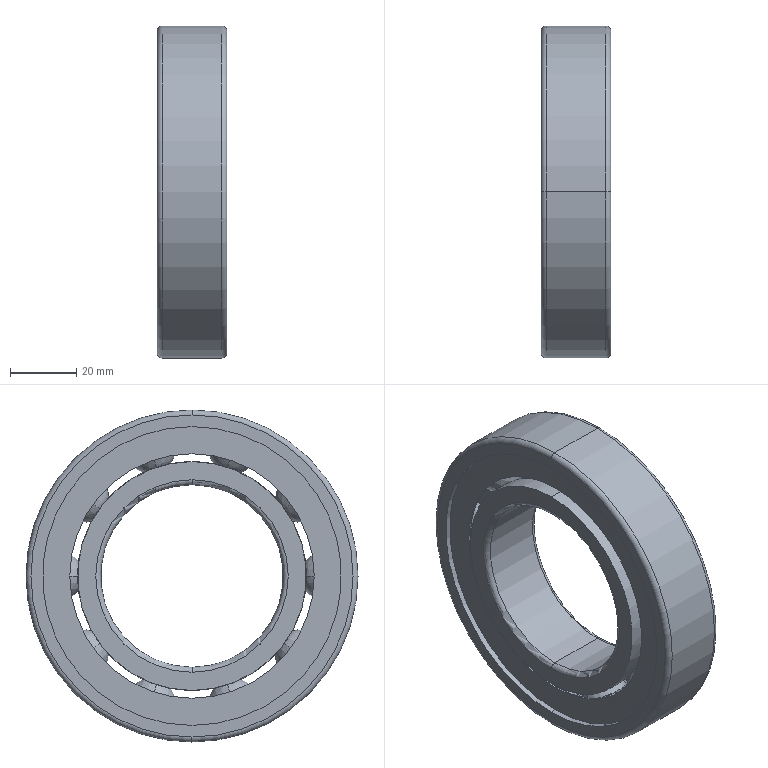Part | SolidWorks | features Revolution 6, CirPattern 2, RevCut 2, MirrorPattern 1 | 1 solid | 173 faces | box 21 x 100 x 100 mm | volume 73176 mm3 | sphere 80 | torus 41 | plane 28 | cylinder 24 | commonest cylinder face diameters 90 x8 68.9 x4 73.615 x4 55 x2 75.521 x2 83.379 x2